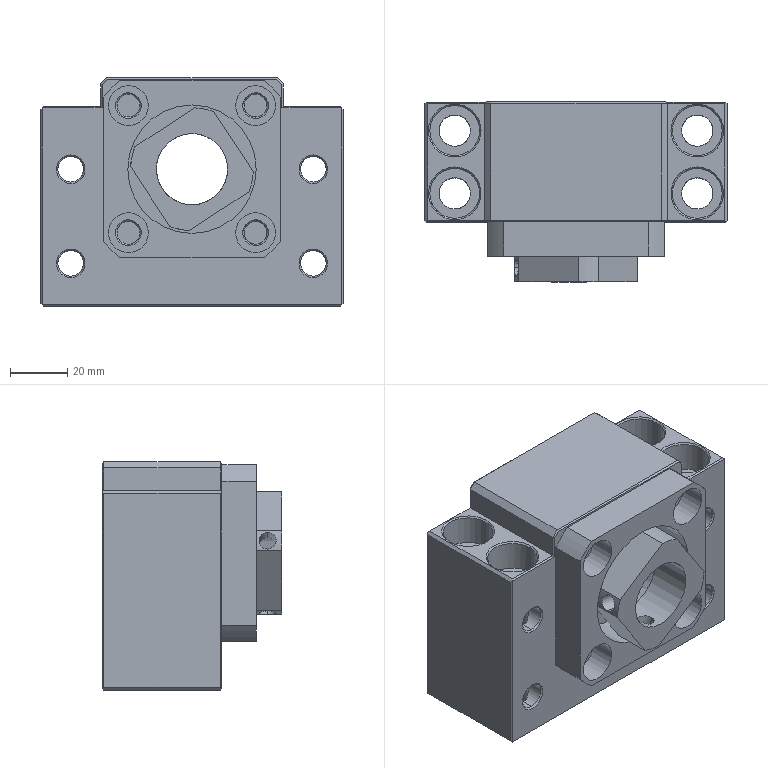Part | STEP file | bearing support block BK25 | 7 solids | 222 faces | box 106 x 63 x 80 mm | volume 295057 mm3 | cylinder 106 | plane 72 | cone 40 | spline 4 | commonest cylinder face diameters 9 x32 25 x10 8 x8 11 x8 14 x8 17.5 x8